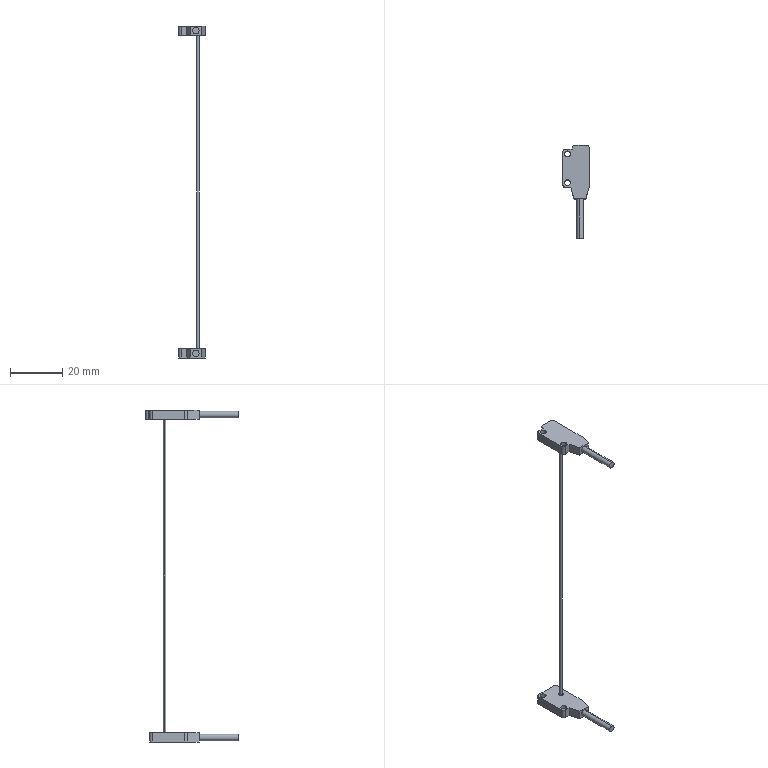Part | STEP file | Through-beam ultra-thin photoelectric switch EX-11A_120 | 2 solids | 50 faces | box 10 x 35.5 x 127 mm | volume 1412 mm3 | cylinder 25 | plane 25 | commonest cylinder face diameters 2 x11 2.2 x8 2.5 x4 1 x2